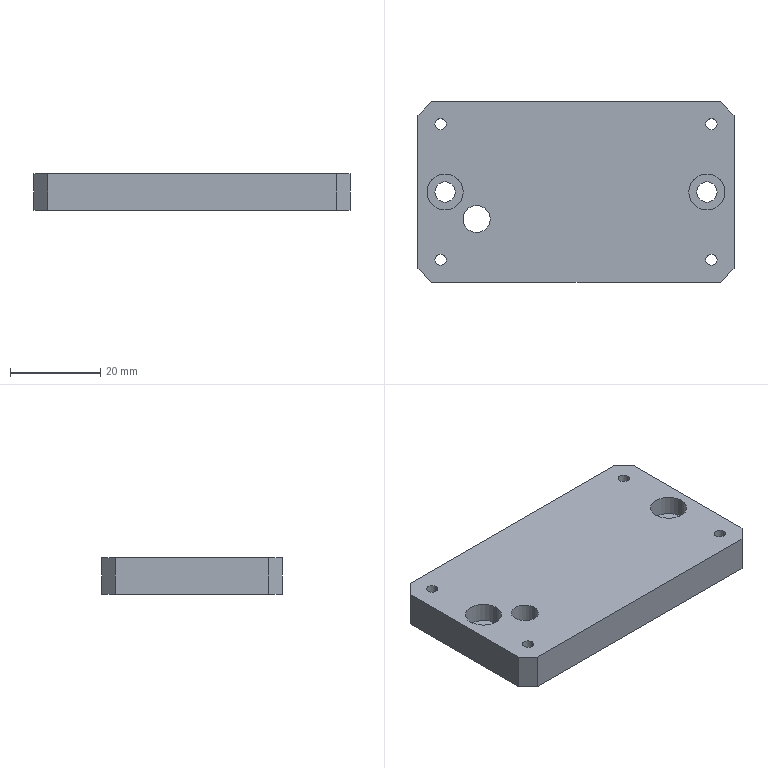Part | STEP file | 11-FG-Z00611 | 1 solid | 36 faces | box 70 x 40 x 8 mm | volume 21065 mm3 | cylinder 22 | plane 14 | commonest cylinder face diameters 2.5 x8 4.5 x4 8 x4 10 x4 6 x2
STEP:
#1=CARTESIAN_POINT('',(-25.,-6.,0.));
#2=VERTEX_POINT('',#1);
#3=CARTESIAN_POINT('',(-19.,-6.,0.));
#4=VERTEX_POINT('',#3);
#5=CARTESIAN_POINT('',(-22.,-6.,0.));
#6=DIRECTION('',(0.,0.,1.));
#7=DIRECTION('',(1.,0.,0.));
#8=AXIS2_PLACEMENT_3D('',#5,#6,#7);
#9=CIRCLE('',#8,3.);
#10=EDGE_CURVE('',#2,#4,#9,.T.);
#11=ORIENTED_EDGE('',*,*,#10,.F.);
#12=CARTESIAN_POINT('',(-25.,-6.,8.));
#13=VERTEX_POINT('',#12);
#14=CARTESIAN_POINT('',(-25.,-6.,-2.));
#15=DIRECTION('',(0.,0.,1.));
#16=VECTOR('',#15,1000.);
#17=LINE('',#14,#16);
#18=EDGE_CURVE('',#2,#13,#17,.T.);
#19=ORIENTED_EDGE('',*,*,#18,.T.);
#20=CARTESIAN_POINT('',(-19.,-6.,8.));
#21=VERTEX_POINT('',#20);
#22=CARTESIAN_POINT('',(-22.,-6.,8.));
#23=DIRECTION('',(0.,0.,1.));
#24=DIRECTION('',(1.,0.,0.));
#25=AXIS2_PLACEMENT_3D('',#22,#23,#24);
#26=CIRCLE('',#25,3.);
#27=EDGE_CURVE('',#13,#21,#26,.T.);
#28=ORIENTED_EDGE('',*,*,#27,.T.);
#29=CARTESIAN_POINT('',(-19.,-6.,-2.));
#30=DIRECTION('',(0.,0.,1.));
#31=VECTOR('',#30,1000.);
#32=LINE('',#29,#31);
#33=EDGE_CURVE('',#4,#21,#32,.T.);
#34=ORIENTED_EDGE('',*,*,#33,.F.);
#35=EDGE_LOOP('',(#11,#19,#28,#34));
#36=FACE_OUTER_BOUND('',#35,.T.);
#37=CARTESIAN_POINT('',(-22.,-6.,-2.));
#38=DIRECTION('',(0.,0.,1.));
#39=DIRECTION('',(1.,0.,0.));
#40=AXIS2_PLACEMENT_3D('',#37,#38,#39);
#41=CYLINDRICAL_SURFACE('',#40,3.);
#42=ADVANCED_FACE('',(#36),#41,.F.);
#43=CARTESIAN_POINT('',(-31.25,15.,0.));
#44=VERTEX_POINT('',#43);
#45=CARTESIAN_POINT('',(-28.75,15.,0.));
#46=VERTEX_POINT('',#45);
#47=CARTESIAN_POINT('',(-30.,15.,0.));
#48=DIRECTION('',(0.,0.,1.));
#49=DIRECTION('',(1.,0.,0.));
#50=AXIS2_PLACEMENT_3D('',#47,#48,#49);
#51=CIRCLE('',#50,1.25);
#52=EDGE_CURVE('',#44,#46,#51,.T.);
#53=ORIENTED_EDGE('',*,*,#52,.F.);
#54=CARTESIAN_POINT('',(-31.25,15.,8.));
#55=VERTEX_POINT('',#54);
#56=CARTESIAN_POINT('',(-31.25,15.,8.));
#57=DIRECTION('',(0.,0.,1.));
#58=VECTOR('',#57,1000.);
#59=LINE('',#56,#58);
#60=EDGE_CURVE('',#44,#55,#59,.T.);
#61=ORIENTED_EDGE('',*,*,#60,.T.);
#62=CARTESIAN_POINT('',(-28.75,15.,8.));
#63=VERTEX_POINT('',#62);
#64=CARTESIAN_POINT('',(-30.,15.,8.));
#65=DIRECTION('',(0.,0.,1.));
#66=DIRECTION('',(1.,0.,0.));
#67=AXIS2_PLACEMENT_3D('',#64,#65,#66);
#68=CIRCLE('',#67,1.25);
#69=EDGE_CURVE('',#55,#63,#68,.T.);
#70=ORIENTED_EDGE('',*,*,#69,.T.);
#71=CARTESIAN_POINT('',(-28.75,15.,8.));
#72=DIRECTION('',(0.,0.,1.));
#73=VECTOR('',#72,1000.);
#74=LINE('',#71,#73);
#75=EDGE_CURVE('',#46,#63,#74,.T.);
#76=ORIENTED_EDGE('',*,*,#75,.F.);
#77=EDGE_LOOP('',(#53,#61,#70,#76));
#78=FACE_OUTER_BOUND('',#77,.T.);
#79=CARTESIAN_POINT('',(-30.,15.,8.));
#80=DIRECTION('',(0.,0.,1.));
#81=DIRECTION('',(1.,0.,0.));
#82=AXIS2_PLACEMENT_3D('',#79,#80,#81);
#83=CYLINDRICAL_SURFACE('',#82,1.25);
#84=ADVANCED_FACE('',(#78),#83,.F.);
#85=CARTESIAN_POINT('',(-31.25,-15.,0.));
#86=VERTEX_POINT('',#85);
#87=CARTESIAN_POINT('',(-28.75,-15.,0.));
#88=VERTEX_POINT('',#87);
#89=CARTESIAN_POINT('',(-30.,-15.,0.));
#90=DIRECTION('',(0.,0.,1.));
#91=DIRECTION('',(1.,0.,0.));
#92=AXIS2_PLACEMENT_3D('',#89,#90,#91);
#93=CIRCLE('',#92,1.25);
#94=EDGE_CURVE('',#86,#88,#93,.T.);
#95=ORIENTED_EDGE('',*,*,#94,.F.);
#96=CARTESIAN_POINT('',(-31.25,-15.,8.));
#97=VERTEX_POINT('',#96);
#98=CARTESIAN_POINT('',(-31.25,-15.,8.));
#99=DIRECTION('',(0.,0.,1.));
#100=VECTOR('',#99,1000.);
#101=LINE('',#98,#100);
#102=EDGE_CURVE('',#86,#97,#101,.T.);
#103=ORIENTED_EDGE('',*,*,#102,.T.);
#104=CARTESIAN_POINT('',(-28.75,-15.,8.));
#105=VERTEX_POINT('',#104);
#106=CARTESIAN_POINT('',(-30.,-15.,8.));
#107=DIRECTION('',(0.,0.,1.));
#108=DIRECTION('',(1.,0.,0.));
#109=AXIS2_PLACEMENT_3D('',#106,#107,#108);
#110=CIRCLE('',#109,1.25);
#111=EDGE_CURVE('',#97,#105,#110,.T.);
#112=ORIENTED_EDGE('',*,*,#111,.T.);
#113=CARTESIAN_POINT('',(-28.75,-15.,8.));
#114=DIRECTION('',(0.,0.,1.));
#115=VECTOR('',#114,1000.);
#116=LINE('',#113,#115);
#117=EDGE_CURVE('',#88,#105,#116,.T.);
#118=ORIENTED_EDGE('',*,*,#117,.F.);
#119=EDGE_LOOP('',(#95,#103,#112,#118));
#120=FACE_OUTER_BOUND('',#119,.T.);
#121=CARTESIAN_POINT('',(-30.,-15.,8.));
#122=DIRECTION('',(0.,0.,1.));
#123=DIRECTION('',(1.,0.,0.));
#124=AXIS2_PLACEMENT_3D('',#121,#122,#123);
#125=CYLINDRICAL_SURFACE('',#124,1.25);
#126=ADVANCED_FACE('',(#120),#125,.F.);
#127=CARTESIAN_POINT('',(28.75,-15.,0.));
#128=VERTEX_POINT('',#127);
#129=CARTESIAN_POINT('',(31.25,-15.,0.));
#130=VERTEX_POINT('',#129);
#131=CARTESIAN_POINT('',(30.,-15.,0.));
#132=DIRECTION('',(0.,0.,1.));
#133=DIRECTION('',(1.,0.,0.));
#134=AXIS2_PLACEMENT_3D('',#131,#132,#133);
#135=CIRCLE('',#134,1.25);
#136=EDGE_CURVE('',#128,#130,#135,.T.);
#137=ORIENTED_EDGE('',*,*,#136,.F.);
#138=CARTESIAN_POINT('',(28.75,-15.,8.));
#139=VERTEX_POINT('',#138);
#140=CARTESIAN_POINT('',(28.75,-15.,8.));
#141=DIRECTION('',(0.,0.,1.));
#142=VECTOR('',#141,1000.);
#143=LINE('',#140,#142);
#144=EDGE_CURVE('',#128,#139,#143,.T.);
#145=ORIENTED_EDGE('',*,*,#144,.T.);
#146=CARTESIAN_POINT('',(31.25,-15.,8.));
#147=VERTEX_POINT('',#146);
#148=CARTESIAN_POINT('',(30.,-15.,8.));
#149=DIRECTION('',(0.,0.,1.));
#150=DIRECTION('',(1.,0.,0.));
#151=AXIS2_PLACEMENT_3D('',#148,#149,#150);
#152=CIRCLE('',#151,1.25);
#153=EDGE_CURVE('',#139,#147,#152,.T.);
#154=ORIENTED_EDGE('',*,*,#153,.T.);
#155=CARTESIAN_POINT('',(31.25,-15.,8.));
#156=DIRECTION('',(0.,0.,1.));
#157=VECTOR('',#156,1000.);
#158=LINE('',#155,#157);
#159=EDGE_CURVE('',#130,#147,#158,.T.);
#160=ORIENTED_EDGE('',*,*,#159,.F.);
#161=EDGE_LOOP('',(#137,#145,#154,#160));
#162=FACE_OUTER_BOUND('',#161,.T.);
#163=CARTESIAN_POINT('',(30.,-15.,8.));
#164=DIRECTION('',(0.,0.,1.));
#165=DIRECTION('',(1.,0.,0.));
#166=AXIS2_PLACEMENT_3D('',#163,#164,#165);
#167=CYLINDRICAL_SURFACE('',#166,1.25);
#168=ADVANCED_FACE('',(#162),#167,.F.);
#169=CARTESIAN_POINT('',(28.75,15.,0.));
#170=VERTEX_POINT('',#169);
#171=CARTESIAN_POINT('',(31.25,15.,0.));
#172=VERTEX_POINT('',#171);
#173=CARTESIAN_POINT('',(30.,15.,0.));
#174=DIRECTION('',(0.,0.,1.));
#175=DIRECTION('',(1.,0.,0.));
#176=AXIS2_PLACEMENT_3D('',#173,#174,#175);
#177=CIRCLE('',#176,1.25);
#178=EDGE_CURVE('',#170,#172,#177,.T.);
#179=ORIENTED_EDGE('',*,*,#178,.F.);
#180=CARTESIAN_POINT('',(28.75,15.,8.));
#181=VERTEX_POINT('',#180);
#182=CARTESIAN_POINT('',(28.75,15.,8.));
#183=DIRECTION('',(0.,0.,1.));
#184=VECTOR('',#183,1000.);
#185=LINE('',#182,#184);
#186=EDGE_CURVE('',#170,#181,#185,.T.);
#187=ORIENTED_EDGE('',*,*,#186,.T.);
#188=CARTESIAN_POINT('',(31.25,15.,8.));
#189=VERTEX_POINT('',#188);
#190=CARTESIAN_POINT('',(30.,15.,8.));
#191=DIRECTION('',(0.,0.,1.));
#192=DIRECTION('',(1.,0.,0.));
#193=AXIS2_PLACEMENT_3D('',#190,#191,#192);
#194=CIRCLE('',#193,1.25);
#195=EDGE_CURVE('',#181,#189,#194,.T.);
#196=ORIENTED_EDGE('',*,*,#195,.T.);
#197=CARTESIAN_POINT('',(31.25,15.,8.));
#198=DIRECTION('',(0.,0.,1.));
#199=VECTOR('',#198,1000.);
#200=LINE('',#197,#199);
#201=EDGE_CURVE('',#172,#189,#200,.T.);
#202=ORIENTED_EDGE('',*,*,#201,.F.);
#203=EDGE_LOOP('',(#179,#187,#196,#202));
#204=FACE_OUTER_BOUND('',#203,.T.);
#205=CARTESIAN_POINT('',(30.,15.,8.));
#206=DIRECTION('',(0.,0.,1.));
#207=DIRECTION('',(1.,0.,0.));
#208=AXIS2_PLACEMENT_3D('',#205,#206,#207);
#209=CYLINDRICAL_SURFACE('',#208,1.25);
#210=ADVANCED_FACE('',(#204),#209,.F.);
#211=CARTESIAN_POINT('',(34.,0.,2.));
#212=VERTEX_POINT('',#211);
#213=CARTESIAN_POINT('',(24.,0.,2.));
#214=VERTEX_POINT('',#213);
#215=CARTESIAN_POINT('',(29.,0.,2.));
#216=DIRECTION('',(0.,0.,-1.));
#217=DIRECTION('',(-1.,0.,0.));
#218=AXIS2_PLACEMENT_3D('',#215,#216,#217);
#219=CIRCLE('',#218,5.);
#220=EDGE_CURVE('',#212,#214,#219,.T.);
#221=ORIENTED_EDGE('',*,*,#220,.F.);
#222=CARTESIAN_POINT('',(34.,0.,0.));
#223=VERTEX_POINT('',#222);
#224=CARTESIAN_POINT('',(34.,0.,2.));
#225=DIRECTION('',(0.,0.,-1.));
#226=VECTOR('',#225,1000.);
#227=LINE('',#224,#226);
#228=EDGE_CURVE('',#212,#223,#227,.T.);
#229=ORIENTED_EDGE('',*,*,#228,.T.);
#230=CARTESIAN_POINT('',(24.,0.,0.));
#231=VERTEX_POINT('',#230);
#232=CARTESIAN_POINT('',(29.,0.,0.));
#233=DIRECTION('',(0.,0.,-1.));
#234=DIRECTION('',(-1.,0.,0.));
#235=AXIS2_PLACEMENT_3D('',#232,#233,#234);
#236=CIRCLE('',#235,5.);
#237=EDGE_CURVE('',#223,#231,#236,.T.);
#238=ORIENTED_EDGE('',*,*,#237,.T.);
#239=CARTESIAN_POINT('',(24.,0.,2.));
#240=DIRECTION('',(0.,0.,-1.));
#241=VECTOR('',#240,1000.);
#242=LINE('',#239,#241);
#243=EDGE_CURVE('',#214,#231,#242,.T.);
#244=ORIENTED_EDGE('',*,*,#243,.F.);
#245=EDGE_LOOP('',(#221,#229,#238,#244));
#246=FACE_OUTER_BOUND('',#245,.T.);
#247=CARTESIAN_POINT('',(29.,0.,2.));
#248=DIRECTION('',(0.,0.,-1.));
#249=DIRECTION('',(-1.,0.,0.));
#250=AXIS2_PLACEMENT_3D('',#247,#248,#249);
#251=CYLINDRICAL_SURFACE('',#250,5.);
#252=ADVANCED_FACE('',(#246),#251,.F.);
#253=CARTESIAN_POINT('',(-24.,0.,2.));
#254=VERTEX_POINT('',#253);
#255=CARTESIAN_POINT('',(-34.,0.,2.));
#256=VERTEX_POINT('',#255);
#257=CARTESIAN_POINT('',(-29.,0.,2.));
#258=DIRECTION('',(0.,0.,-1.));
#259=DIRECTION('',(-1.,0.,0.));
#260=AXIS2_PLACEMENT_3D('',#257,#258,#259);
#261=CIRCLE('',#260,5.);
#262=EDGE_CURVE('',#254,#256,#261,.T.);
#263=ORIENTED_EDGE('',*,*,#262,.F.);
#264=CARTESIAN_POINT('',(-24.,0.,0.));
#265=VERTEX_POINT('',#264);
#266=CARTESIAN_POINT('',(-24.,0.,2.));
#267=DIRECTION('',(0.,0.,-1.));
#268=VECTOR('',#267,1000.);
#269=LINE('',#266,#268);
#270=EDGE_CURVE('',#254,#265,#269,.T.);
#271=ORIENTED_EDGE('',*,*,#270,.T.);
#272=CARTESIAN_POINT('',(-34.,0.,0.));
#273=VERTEX_POINT('',#272);
#274=CARTESIAN_POINT('',(-29.,0.,0.));
#275=DIRECTION('',(0.,0.,-1.));
#276=DIRECTION('',(-1.,0.,0.));
#277=AXIS2_PLACEMENT_3D('',#274,#275,#276);
#278=CIRCLE('',#277,5.);
#279=EDGE_CURVE('',#265,#273,#278,.T.);
#280=ORIENTED_EDGE('',*,*,#279,.T.);
#281=CARTESIAN_POINT('',(-34.,0.,2.));
#282=DIRECTION('',(0.,0.,-1.));
#283=VECTOR('',#282,1000.);
#284=LINE('',#281,#283);
#285=EDGE_CURVE('',#256,#273,#284,.T.);
#286=ORIENTED_EDGE('',*,*,#285,.F.);
#287=EDGE_LOOP('',(#263,#271,#280,#286));
#288=FACE_OUTER_BOUND('',#287,.T.);
#289=CARTESIAN_POINT('',(-29.,0.,2.));
#290=DIRECTION('',(0.,0.,-1.));
#291=DIRECTION('',(-1.,0.,0.));
#292=AXIS2_PLACEMENT_3D('',#289,#290,#291);
#293=CYLINDRICAL_SURFACE('',#292,5.);
#294=ADVANCED_FACE('',(#288),#293,.F.);
#295=CARTESIAN_POINT('',(-33.,0.,3.6));
#296=VERTEX_POINT('',#295);
#297=CARTESIAN_POINT('',(-25.,0.,3.6));
#298=VERTEX_POINT('',#297);
#299=CARTESIAN_POINT('',(-29.,0.,3.6));
#300=DIRECTION('',(0.,0.,1.));
#301=DIRECTION('',(1.,0.,0.));
#302=AXIS2_PLACEMENT_3D('',#299,#300,#301);
#303=CIRCLE('',#302,4.);
#304=EDGE_CURVE('',#296,#298,#303,.T.);
#305=ORIENTED_EDGE('',*,*,#304,.F.);
#306=CARTESIAN_POINT('',(-33.,0.,8.));
#307=VERTEX_POINT('',#306);
#308=CARTESIAN_POINT('',(-33.,0.,8.));
#309=DIRECTION('',(0.,0.,1.));
#310=VECTOR('',#309,1000.);
#311=LINE('',#308,#310);
#312=EDGE_CURVE('',#296,#307,#311,.T.);
#313=ORIENTED_EDGE('',*,*,#312,.T.);
#314=CARTESIAN_POINT('',(-25.,0.,8.));
#315=VERTEX_POINT('',#314);
#316=CARTESIAN_POINT('',(-29.,0.,8.));
#317=DIRECTION('',(0.,0.,1.));
#318=DIRECTION('',(1.,0.,0.));
#319=AXIS2_PLACEMENT_3D('',#316,#317,#318);
#320=CIRCLE('',#319,4.);
#321=EDGE_CURVE('',#307,#315,#320,.T.);
#322=ORIENTED_EDGE('',*,*,#321,.T.);
#323=CARTESIAN_POINT('',(-25.,0.,8.));
#324=DIRECTION('',(0.,0.,1.));
#325=VECTOR('',#324,1000.);
#326=LINE('',#323,#325);
#327=EDGE_CURVE('',#298,#315,#326,.T.);
#328=ORIENTED_EDGE('',*,*,#327,.F.);
#329=EDGE_LOOP('',(#305,#313,#322,#328));
#330=FACE_OUTER_BOUND('',#329,.T.);
#331=CARTESIAN_POINT('',(-29.,0.,8.));
#332=DIRECTION('',(0.,0.,1.));
#333=DIRECTION('',(1.,0.,0.));
#334=AXIS2_PLACEMENT_3D('',#331,#332,#333);
#335=CYLINDRICAL_SURFACE('',#334,4.);
#336=ADVANCED_FACE('',(#330),#335,.F.);
#337=CARTESIAN_POINT('',(25.,0.,3.6));
#338=VERTEX_POINT('',#337);
#339=CARTESIAN_POINT('',(33.,0.,3.6));
#340=VERTEX_POINT('',#339);
#341=CARTESIAN_POINT('',(29.,0.,3.6));
#342=DIRECTION('',(0.,0.,1.));
#343=DIRECTION('',(1.,0.,0.));
#344=AXIS2_PLACEMENT_3D('',#341,#342,#343);
#345=CIRCLE('',#344,4.);
#346=EDGE_CURVE('',#338,#340,#345,.T.);
#347=ORIENTED_EDGE('',*,*,#346,.F.);
#348=CARTESIAN_POINT('',(25.,0.,8.));
#349=VERTEX_POINT('',#348);
#350=CARTESIAN_POINT('',(25.,0.,8.));
#351=DIRECTION('',(0.,0.,1.));
#352=VECTOR('',#351,1000.);
#353=LINE('',#350,#352);
#354=EDGE_CURVE('',#338,#349,#353,.T.);
#355=ORIENTED_EDGE('',*,*,#354,.T.);
#356=CARTESIAN_POINT('',(33.,0.,8.));
#357=VERTEX_POINT('',#356);
#358=CARTESIAN_POINT('',(29.,0.,8.));
#359=DIRECTION('',(0.,0.,1.));
#360=DIRECTION('',(1.,0.,0.));
#361=AXIS2_PLACEMENT_3D('',#358,#359,#360);
#362=CIRCLE('',#361,4.);
#363=EDGE_CURVE('',#349,#357,#362,.T.);
#364=ORIENTED_EDGE('',*,*,#363,.T.);
#365=CARTESIAN_POINT('',(33.,0.,8.));
#366=DIRECTION('',(0.,0.,1.));
#367=VECTOR('',#366,1000.);
#368=LINE('',#365,#367);
#369=EDGE_CURVE('',#340,#357,#368,.T.);
#370=ORIENTED_EDGE('',*,*,#369,.F.);
#371=EDGE_LOOP('',(#347,#355,#364,#370));
#372=FACE_OUTER_BOUND('',#371,.T.);
#373=CARTESIAN_POINT('',(29.,0.,8.));
#374=DIRECTION('',(0.,0.,1.));
#375=DIRECTION('',(1.,0.,0.));
#376=AXIS2_PLACEMENT_3D('',#373,#374,#375);
#377=CYLINDRICAL_SURFACE('',#376,4.);
#378=ADVANCED_FACE('',(#372),#377,.F.);
#379=CARTESIAN_POINT('',(-31.25,0.,2.));
#380=VERTEX_POINT('',#379);
#381=CARTESIAN_POINT('',(-26.75,0.,2.));
#382=VERTEX_POINT('',#381);
#383=CARTESIAN_POINT('',(-29.,0.,2.));
#384=DIRECTION('',(0.,0.,1.));
#385=DIRECTION('',(-1.,0.,0.));
#386=AXIS2_PLACEMENT_3D('',#383,#384,#385);
#387=CIRCLE('',#386,2.25);
#388=EDGE_CURVE('',#380,#382,#387,.T.);
#389=ORIENTED_EDGE('',*,*,#388,.F.);
#390=CARTESIAN_POINT('',(-31.25,0.,3.6));
#391=VERTEX_POINT('',#390);
#392=CARTESIAN_POINT('',(-31.25,0.,8.));
#393=DIRECTION('',(0.,0.,1.));
#394=VECTOR('',#393,1000.);
#395=LINE('',#392,#394);
#396=EDGE_CURVE('',#380,#391,#395,.T.);
#397=ORIENTED_EDGE('',*,*,#396,.T.);
#398=CARTESIAN_POINT('',(-26.75,0.,3.6));
#399=VERTEX_POINT('',#398);
#400=CARTESIAN_POINT('',(-29.,0.,3.6));
#401=DIRECTION('',(0.,0.,1.));
#402=DIRECTION('',(1.,0.,0.));
#403=AXIS2_PLACEMENT_3D('',#400,#401,#402);
#404=CIRCLE('',#403,2.25);
#405=EDGE_CURVE('',#391,#399,#404,.T.);
#406=ORIENTED_EDGE('',*,*,#405,.T.);
#407=CARTESIAN_POINT('',(-26.75,0.,8.));
#408=DIRECTION('',(0.,0.,1.));
#409=VECTOR('',#408,1000.);
#410=LINE('',#407,#409);
#411=EDGE_CURVE('',#382,#399,#410,.T.);
#412=ORIENTED_EDGE('',*,*,#411,.F.);
#413=EDGE_LOOP('',(#389,#397,#406,#412));
#414=FACE_OUTER_BOUND('',#413,.T.);
#415=CARTESIAN_POINT('',(-29.,0.,8.));
#416=DIRECTION('',(0.,0.,1.));
#417=DIRECTION('',(1.,0.,0.));
#418=AXIS2_PLACEMENT_3D('',#415,#416,#417);
#419=CYLINDRICAL_SURFACE('',#418,2.25);
#420=ADVANCED_FACE('',(#414),#419,.F.);
#421=CARTESIAN_POINT('',(26.75,0.,2.));
#422=VERTEX_POINT('',#421);
#423=CARTESIAN_POINT('',(31.25,0.,2.));
#424=VERTEX_POINT('',#423);
#425=CARTESIAN_POINT('',(29.,0.,2.));
#426=DIRECTION('',(0.,0.,1.));
#427=DIRECTION('',(-1.,0.,0.));
#428=AXIS2_PLACEMENT_3D('',#425,#426,#427);
#429=CIRCLE('',#428,2.25);
#430=EDGE_CURVE('',#422,#424,#429,.T.);
#431=ORIENTED_EDGE('',*,*,#430,.F.);
#432=CARTESIAN_POINT('',(26.75,0.,3.6));
#433=VERTEX_POINT('',#432);
#434=CARTESIAN_POINT('',(26.75,0.,8.));
#435=DIRECTION('',(0.,0.,1.));
#436=VECTOR('',#435,1000.);
#437=LINE('',#434,#436);
#438=EDGE_CURVE('',#422,#433,#437,.T.);
#439=ORIENTED_EDGE('',*,*,#438,.T.);
#440=CARTESIAN_POINT('',(31.25,0.,3.6));
#441=VERTEX_POINT('',#440);
#442=CARTESIAN_POINT('',(29.,0.,3.6));
#443=DIRECTION('',(0.,0.,1.));
#444=DIRECTION('',(1.,0.,0.));
#445=AXIS2_PLACEMENT_3D('',#442,#443,#444);
#446=CIRCLE('',#445,2.25);
#447=EDGE_CURVE('',#433,#441,#446,.T.);
#448=ORIENTED_EDGE('',*,*,#447,.T.);
#449=CARTESIAN_POINT('',(31.25,0.,8.));
#450=DIRECTION('',(0.,0.,1.));
#451=VECTOR('',#450,1000.);
#452=LINE('',#449,#451);
#453=EDGE_CURVE('',#424,#441,#452,.T.);
#454=ORIENTED_EDGE('',*,*,#453,.F.);
#455=EDGE_LOOP('',(#431,#439,#448,#454));
#456=FACE_OUTER_BOUND('',#455,.T.);
#457=CARTESIAN_POINT('',(29.,0.,8.));
#458=DIRECTION('',(0.,0.,1.));
#459=DIRECTION('',(1.,0.,0.));
#460=AXIS2_PLACEMENT_3D('',#457,#458,#459);
#461=CYLINDRICAL_SURFACE('',#460,2.25);
#462=ADVANCED_FACE('',(#456),#461,.F.);
#463=ORIENTED_EDGE('',*,*,#438,.F.);
#464=CARTESIAN_POINT('',(29.,0.,2.));
#465=DIRECTION('',(0.,0.,1.));
#466=DIRECTION('',(-1.,0.,0.));
#467=AXIS2_PLACEMENT_3D('',#464,#465,#466);
#468=CIRCLE('',#467,2.25);
#469=EDGE_CURVE('',#424,#422,#468,.T.);
#470=ORIENTED_EDGE('',*,*,#469,.F.);
#471=ORIENTED_EDGE('',*,*,#453,.T.);
#472=CARTESIAN_POINT('',(29.,0.,3.6));
#473=DIRECTION('',(0.,0.,1.));
#474=DIRECTION('',(1.,0.,0.));
#475=AXIS2_PLACEMENT_3D('',#472,#473,#474);
#476=CIRCLE('',#475,2.25);
#477=EDGE_CURVE('',#441,#433,#476,.T.);
#478=ORIENTED_EDGE('',*,*,#477,.T.);
#479=EDGE_LOOP('',(#463,#470,#471,#478));
#480=FACE_OUTER_BOUND('',#479,.T.);
#481=CARTESIAN_POINT('',(29.,0.,8.));
#482=DIRECTION('',(0.,0.,1.));
#483=DIRECTION('',(1.,0.,0.));
#484=AXIS2_PLACEMENT_3D('',#481,#482,#483);
#485=CYLINDRICAL_SURFACE('',#484,2.25);
#486=ADVANCED_FACE('',(#480),#485,.F.);
#487=ORIENTED_EDGE('',*,*,#396,.F.);
#488=CARTESIAN_POINT('',(-29.,0.,2.));
#489=DIRECTION('',(0.,0.,1.));
#490=DIRECTION('',(-1.,0.,0.));
#491=AXIS2_PLACEMENT_3D('',#488,#489,#490);
#492=CIRCLE('',#491,2.25);
#493=EDGE_CURVE('',#382,#380,#492,.T.);
#494=ORIENTED_EDGE('',*,*,#493,.F.);
#495=ORIENTED_EDGE('',*,*,#411,.T.);
#496=CARTESIAN_POINT('',(-29.,0.,3.6));
#497=DIRECTION('',(0.,0.,1.));
#498=DIRECTION('',(1.,0.,0.));
#499=AXIS2_PLACEMENT_3D('',#496,#497,#498);
#500=CIRCLE('',#499,2.25);
#501=EDGE_CURVE('',#399,#391,#500,.T.);
#502=ORIENTED_EDGE('',*,*,#501,.T.);
#503=EDGE_LOOP('',(#487,#494,#495,#502));
#504=FACE_OUTER_BOUND('',#503,.T.);
#505=CARTESIAN_POINT('',(-29.,0.,8.));
#506=DIRECTION('',(0.,0.,1.));
#507=DIRECTION('',(1.,0.,0.));
#508=AXIS2_PLACEMENT_3D('',#505,#506,#507);
#509=CYLINDRICAL_SURFACE('',#508,2.25);
#510=ADVANCED_FACE('',(#504),#509,.F.);
#511=CARTESIAN_POINT('',(35.,-17.,8.));
#512=VERTEX_POINT('',#511);
#513=CARTESIAN_POINT('',(35.,17.,8.));
#514=VERTEX_POINT('',#513);
#515=CARTESIAN_POINT('',(35.,20.,8.));
#516=DIRECTION('',(0.,1.,0.));
#517=VECTOR('',#516,1000.);
#518=LINE('',#515,#517);
#519=EDGE_CURVE('',#512,#514,#518,.T.);
#520=ORIENTED_EDGE('',*,*,#519,.F.);
#521=CARTESIAN_POINT('',(35.,-17.,0.));
#522=VERTEX_POINT('',#521);
#523=CARTESIAN_POINT('',(35.,-17.,8.));
#524=DIRECTION('',(0.,0.,-1.));
#525=VECTOR('',#524,1000.);
#526=LINE('',#523,#525);
#527=EDGE_CURVE('',#512,#522,#526,.T.);
#528=ORIENTED_EDGE('',*,*,#527,.T.);
#529=CARTESIAN_POINT('',(35.,17.,0.));
#530=VERTEX_POINT('',#529);
#531=CARTESIAN_POINT('',(35.,20.,0.));
#532=DIRECTION('',(0.,1.,0.));
#533=VECTOR('',#532,1000.);
#534=LINE('',#531,#533);
#535=EDGE_CURVE('',#522,#530,#534,.T.);
#536=ORIENTED_EDGE('',*,*,#535,.T.);
#537=CARTESIAN_POINT('',(35.,17.,8.));
#538=DIRECTION('',(0.,0.,1.));
#539=VECTOR('',#538,1000.);
#540=LINE('',#537,#539);
#541=EDGE_CURVE('',#530,#514,#540,.T.);
#542=ORIENTED_EDGE('',*,*,#541,.T.);
#543=EDGE_LOOP('',(#520,#528,#536,#542));
#544=FACE_OUTER_BOUND('',#543,.T.);
#545=CARTESIAN_POINT('',(35.,20.,8.));
#546=DIRECTION('',(-1.,0.,0.));
#547=DIRECTION('',(0.,-1.,0.));
#548=AXIS2_PLACEMENT_3D('',#545,#546,#547);
#549=PLANE('',#548);
#550=ADVANCED_FACE('',(#544),#549,.F.);
#551=CARTESIAN_POINT('',(32.,20.,8.));
#552=VERTEX_POINT('',#551);
#553=CARTESIAN_POINT('',(-32.,20.,8.));
#554=VERTEX_POINT('',#553);
#555=CARTESIAN_POINT('',(-35.,20.,8.));
#556=DIRECTION('',(-1.,0.,0.));
#557=VECTOR('',#556,1000.);
#558=LINE('',#555,#557);
#559=EDGE_CURVE('',#552,#554,#558,.T.);
#560=ORIENTED_EDGE('',*,*,#559,.F.);
#561=CARTESIAN_POINT('',(32.,20.,0.));
#562=VERTEX_POINT('',#561);
#563=CARTESIAN_POINT('',(32.,20.,8.));
#564=DIRECTION('',(0.,0.,-1.));
#565=VECTOR('',#564,1000.);
#566=LINE('',#563,#565);
#567=EDGE_CURVE('',#552,#562,#566,.T.);
#568=ORIENTED_EDGE('',*,*,#567,.T.);
#569=CARTESIAN_POINT('',(-32.,20.,0.));
#570=VERTEX_POINT('',#569);
#571=CARTESIAN_POINT('',(-35.,20.,0.));
#572=DIRECTION('',(-1.,0.,0.));
#573=VECTOR('',#572,1000.);
#574=LINE('',#571,#573);
#575=EDGE_CURVE('',#562,#570,#574,.T.);
#576=ORIENTED_EDGE('',*,*,#575,.T.);
#577=CARTESIAN_POINT('',(-32.,20.,8.));
#578=DIRECTION('',(0.,0.,1.));
#579=VECTOR('',#578,1000.);
#580=LINE('',#577,#579);
#581=EDGE_CURVE('',#570,#554,#580,.T.);
#582=ORIENTED_EDGE('',*,*,#581,.T.);
#583=EDGE_LOOP('',(#560,#568,#576,#582));
#584=FACE_OUTER_BOUND('',#583,.T.);
#585=CARTESIAN_POINT('',(-35.,20.,8.));
#586=DIRECTION('',(0.,-1.,0.));
#587=DIRECTION('',(0.,0.,-1.));
#588=AXIS2_PLACEMENT_3D('',#585,#586,#587);
#589=PLANE('',#588);
#590=ADVANCED_FACE('',(#584),#589,.F.);
#591=CARTESIAN_POINT('',(-35.,17.,0.));
#592=VERTEX_POINT('',#591);
#593=CARTESIAN_POINT('',(-35.,-17.,0.));
#594=VERTEX_POINT('',#593);
#595=CARTESIAN_POINT('',(-35.,20.,0.));
#596=DIRECTION('',(0.,-1.,0.));
#597=VECTOR('',#596,1000.);
#598=LINE('',#595,#597);
#599=EDGE_CURVE('',#592,#594,#598,.T.);
#600=ORIENTED_EDGE('',*,*,#599,.T.);
#601=CARTESIAN_POINT('',(-35.,-17.,8.));
#602=VERTEX_POINT('',#601);
#603=CARTESIAN_POINT('',(-35.,-17.,8.));
#604=DIRECTION('',(0.,0.,1.));
#605=VECTOR('',#604,1000.);
#606=LINE('',#603,#605);
#607=EDGE_CURVE('',#594,#602,#606,.T.);
#608=ORIENTED_EDGE('',*,*,#607,.T.);
#609=CARTESIAN_POINT('',(-35.,17.,8.));
#610=VERTEX_POINT('',#609);
#611=CARTESIAN_POINT('',(-35.,20.,8.));
#612=DIRECTION('',(0.,-1.,0.));
#613=VECTOR('',#612,1000.);
#614=LINE('',#611,#613);
#615=EDGE_CURVE('',#610,#602,#614,.T.);
#616=ORIENTED_EDGE('',*,*,#615,.F.);
#617=CARTESIAN_POINT('',(-35.,17.,8.));
#618=DIRECTION('',(0.,0.,-1.));
#619=VECTOR('',#618,1000.);
#620=LINE('',#617,#619);
#621=EDGE_CURVE('',#610,#592,#620,.T.);
#622=ORIENTED_EDGE('',*,*,#621,.T.);
#623=EDGE_LOOP('',(#600,#608,#616,#622));
#624=FACE_OUTER_BOUND('',#623,.T.);
#625=CARTESIAN_POINT('',(-35.,20.,8.));
#626=DIRECTION('',(1.,0.,0.));
#627=DIRECTION('',(0.,1.,0.));
#628=AXIS2_PLACEMENT_3D('',#625,#626,#627);
#629=PLANE('',#628);
#630=ADVANCED_FACE('',(#624),#629,.F.);
#631=CARTESIAN_POINT('',(-32.,-20.,0.));
#632=VERTEX_POINT('',#631);
#633=CARTESIAN_POINT('',(32.,-20.,0.));
#634=VERTEX_POINT('',#633);
#635=CARTESIAN_POINT('',(-35.,-20.,0.));
#636=DIRECTION('',(1.,0.,0.));
#637=VECTOR('',#636,1000.);
#638=LINE('',#635,#637);
#639=EDGE_CURVE('',#632,#634,#638,.T.);
#640=ORIENTED_EDGE('',*,*,#639,.T.);
#641=CARTESIAN_POINT('',(32.,-20.,8.));
#642=VERTEX_POINT('',#641);
#643=CARTESIAN_POINT('',(32.,-20.,8.));
#644=DIRECTION('',(0.,0.,1.));
#645=VECTOR('',#644,1000.);
#646=LINE('',#643,#645);
#647=EDGE_CURVE('',#634,#642,#646,.T.);
#648=ORIENTED_EDGE('',*,*,#647,.T.);
#649=CARTESIAN_POINT('',(-32.,-20.,8.));
#650=VERTEX_POINT('',#649);
#651=CARTESIAN_POINT('',(-35.,-20.,8.));
#652=DIRECTION('',(1.,0.,0.));
#653=VECTOR('',#652,1000.);
#654=LINE('',#651,#653);
#655=EDGE_CURVE('',#650,#642,#654,.T.);
#656=ORIENTED_EDGE('',*,*,#655,.F.);
#657=CARTESIAN_POINT('',(-32.,-20.,8.));
#658=DIRECTION('',(0.,0.,-1.));
#659=VECTOR('',#658,1000.);
#660=LINE('',#657,#659);
#661=EDGE_CURVE('',#650,#632,#660,.T.);
#662=ORIENTED_EDGE('',*,*,#661,.T.);
#663=EDGE_LOOP('',(#640,#648,#656,#662));
#664=FACE_OUTER_BOUND('',#663,.T.);
#665=CARTESIAN_POINT('',(-35.,-20.,8.));
#666=DIRECTION('',(0.,1.,0.));
#667=DIRECTION('',(0.,0.,1.));
#668=AXIS2_PLACEMENT_3D('',#665,#666,#667);
#669=PLANE('',#668);
#670=ADVANCED_FACE('',(#664),#669,.F.);
#671=CARTESIAN_POINT('',(-22.,-6.,8.));
#672=DIRECTION('',(0.,0.,1.));
#673=DIRECTION('',(1.,0.,0.));
#674=AXIS2_PLACEMENT_3D('',#671,#672,#673);
#675=CIRCLE('',#674,3.);
#676=EDGE_CURVE('',#21,#13,#675,.T.);
#677=ORIENTED_EDGE('',*,*,#676,.F.);
#678=ORIENTED_EDGE('',*,*,#27,.F.);
#679=EDGE_LOOP('',(#677,#678));
#680=FACE_BOUND('',#679,.T.);
#681=CARTESIAN_POINT('',(-30.,15.,8.));
#682=DIRECTION('',(0.,0.,1.));
#683=DIRECTION('',(1.,0.,0.));
#684=AXIS2_PLACEMENT_3D('',#681,#682,#683);
#685=CIRCLE('',#684,1.25);
#686=EDGE_CURVE('',#63,#55,#685,.T.);
#687=ORIENTED_EDGE('',*,*,#686,.F.);
#688=ORIENTED_EDGE('',*,*,#69,.F.);
#689=EDGE_LOOP('',(#687,#688));
#690=FACE_BOUND('',#689,.T.);
#691=CARTESIAN_POINT('',(-30.,-15.,8.));
#692=DIRECTION('',(0.,0.,1.));
#693=DIRECTION('',(1.,0.,0.));
#694=AXIS2_PLACEMENT_3D('',#691,#692,#693);
#695=CIRCLE('',#694,1.25);
#696=EDGE_CURVE('',#105,#97,#695,.T.);
#697=ORIENTED_EDGE('',*,*,#696,.F.);
#698=ORIENTED_EDGE('',*,*,#111,.F.);
#699=EDGE_LOOP('',(#697,#698));
#700=FACE_BOUND('',#699,.T.);
#701=CARTESIAN_POINT('',(30.,-15.,8.));
#702=DIRECTION('',(0.,0.,1.));
#703=DIRECTION('',(1.,0.,0.));
#704=AXIS2_PLACEMENT_3D('',#701,#702,#703);
#705=CIRCLE('',#704,1.25);
#706=EDGE_CURVE('',#147,#139,#705,.T.);
#707=ORIENTED_EDGE('',*,*,#706,.F.);
#708=ORIENTED_EDGE('',*,*,#153,.F.);
#709=EDGE_LOOP('',(#707,#708));
#710=FACE_BOUND('',#709,.T.);
#711=CARTESIAN_POINT('',(30.,15.,8.));
#712=DIRECTION('',(0.,0.,1.));
#713=DIRECTION('',(1.,0.,0.));
#714=AXIS2_PLACEMENT_3D('',#711,#712,#713);
#715=CIRCLE('',#714,1.25);
#716=EDGE_CURVE('',#189,#181,#715,.T.);
#717=ORIENTED_EDGE('',*,*,#716,.F.);
#718=ORIENTED_EDGE('',*,*,#195,.F.);
#719=EDGE_LOOP('',(#717,#718));
#720=FACE_BOUND('',#719,.T.);
#721=CARTESIAN_POINT('',(-29.,0.,8.));
#722=DIRECTION('',(0.,0.,1.));
#723=DIRECTION('',(1.,0.,0.));
#724=AXIS2_PLACEMENT_3D('',#721,#722,#723);
#725=CIRCLE('',#724,4.);
#726=EDGE_CURVE('',#315,#307,#725,.T.);
#727=ORIENTED_EDGE('',*,*,#726,.F.);
#728=ORIENTED_EDGE('',*,*,#321,.F.);
#729=EDGE_LOOP('',(#727,#728));
#730=FACE_BOUND('',#729,.T.);
#731=CARTESIAN_POINT('',(29.,0.,8.));
#732=DIRECTION('',(0.,0.,1.));
#733=DIRECTION('',(1.,0.,0.));
#734=AXIS2_PLACEMENT_3D('',#731,#732,#733);
#735=CIRCLE('',#734,4.);
#736=EDGE_CURVE('',#357,#349,#735,.T.);
#737=ORIENTED_EDGE('',*,*,#736,.F.);
#738=ORIENTED_EDGE('',*,*,#363,.F.);
#739=EDGE_LOOP('',(#737,#738));
#740=FACE_BOUND('',#739,.T.);
#741=ORIENTED_EDGE('',*,*,#655,.T.);
#742=CARTESIAN_POINT('',(26.,-26.,8.));
#743=DIRECTION('',(0.7071,0.7071,0.));
#744=VECTOR('',#743,1000.);
#745=LINE('',#742,#744);
#746=EDGE_CURVE('',#642,#512,#745,.T.);
#747=ORIENTED_EDGE('',*,*,#746,.T.);
#748=ORIENTED_EDGE('',*,*,#519,.T.);
#749=CARTESIAN_POINT('',(26.,26.,8.));
#750=DIRECTION('',(-0.7071,0.7071,0.));
#751=VECTOR('',#750,1000.);
#752=LINE('',#749,#751);
#753=EDGE_CURVE('',#514,#552,#752,.T.);
#754=ORIENTED_EDGE('',*,*,#753,.T.);
#755=ORIENTED_EDGE('',*,*,#559,.T.);
#756=CARTESIAN_POINT('',(-26.,26.,8.));
#757=DIRECTION('',(-0.7071,-0.7071,0.));
#758=VECTOR('',#757,1000.);
#759=LINE('',#756,#758);
#760=EDGE_CURVE('',#554,#610,#759,.T.);
#761=ORIENTED_EDGE('',*,*,#760,.T.);
#762=ORIENTED_EDGE('',*,*,#615,.T.);
#763=CARTESIAN_POINT('',(-26.,-26.,8.));
#764=DIRECTION('',(0.7071,-0.7071,0.));
#765=VECTOR('',#764,1000.);
#766=LINE('',#763,#765);
#767=EDGE_CURVE('',#602,#650,#766,.T.);
#768=ORIENTED_EDGE('',*,*,#767,.T.);
#769=EDGE_LOOP('',(#741,#747,#748,#754,#755,#761,#762,#768));
#770=FACE_OUTER_BOUND('',#769,.T.);
#771=CARTESIAN_POINT('',(0.,0.,8.));
#772=DIRECTION('',(0.,0.,1.));
#773=DIRECTION('',(1.,0.,0.));
#774=AXIS2_PLACEMENT_3D('',#771,#772,#773);
#775=PLANE('',#774);
#776=ADVANCED_FACE('',(#680,#690,#700,#710,#720,#730,#740,#770),#775,.T.);
#777=CARTESIAN_POINT('',(-22.,-6.,0.));
#778=DIRECTION('',(0.,0.,1.));
#779=DIRECTION('',(1.,0.,0.));
#780=AXIS2_PLACEMENT_3D('',#777,#778,#779);
#781=CIRCLE('',#780,3.);
#782=EDGE_CURVE('',#4,#2,#781,.T.);
#783=ORIENTED_EDGE('',*,*,#782,.T.);
#784=ORIENTED_EDGE('',*,*,#10,.T.);
#785=EDGE_LOOP('',(#783,#784));
#786=FACE_BOUND('',#785,.T.);
#787=CARTESIAN_POINT('',(-30.,15.,0.));
#788=DIRECTION('',(0.,0.,1.));
#789=DIRECTION('',(1.,0.,0.));
#790=AXIS2_PLACEMENT_3D('',#787,#788,#789);
#791=CIRCLE('',#790,1.25);
#792=EDGE_CURVE('',#46,#44,#791,.T.);
#793=ORIENTED_EDGE('',*,*,#792,.T.);
#794=ORIENTED_EDGE('',*,*,#52,.T.);
#795=EDGE_LOOP('',(#793,#794));
#796=FACE_BOUND('',#795,.T.);
#797=CARTESIAN_POINT('',(-30.,-15.,0.));
#798=DIRECTION('',(0.,0.,1.));
#799=DIRECTION('',(1.,0.,0.));
#800=AXIS2_PLACEMENT_3D('',#797,#798,#799);
#801=CIRCLE('',#800,1.25);
#802=EDGE_CURVE('',#88,#86,#801,.T.);
#803=ORIENTED_EDGE('',*,*,#802,.T.);
#804=ORIENTED_EDGE('',*,*,#94,.T.);
#805=EDGE_LOOP('',(#803,#804));
#806=FACE_BOUND('',#805,.T.);
#807=CARTESIAN_POINT('',(30.,-15.,0.));
#808=DIRECTION('',(0.,0.,1.));
#809=DIRECTION('',(1.,0.,0.));
#810=AXIS2_PLACEMENT_3D('',#807,#808,#809);
#811=CIRCLE('',#810,1.25);
#812=EDGE_CURVE('',#130,#128,#811,.T.);
#813=ORIENTED_EDGE('',*,*,#812,.T.);
#814=ORIENTED_EDGE('',*,*,#136,.T.);
#815=EDGE_LOOP('',(#813,#814));
#816=FACE_BOUND('',#815,.T.);
#817=CARTESIAN_POINT('',(30.,15.,0.));
#818=DIRECTION('',(0.,0.,1.));
#819=DIRECTION('',(1.,0.,0.));
#820=AXIS2_PLACEMENT_3D('',#817,#818,#819);
#821=CIRCLE('',#820,1.25);
#822=EDGE_CURVE('',#172,#170,#821,.T.);
#823=ORIENTED_EDGE('',*,*,#822,.T.);
#824=ORIENTED_EDGE('',*,*,#178,.T.);
#825=EDGE_LOOP('',(#823,#824));
#826=FACE_BOUND('',#825,.T.);
#827=CARTESIAN_POINT('',(29.,0.,0.));
#828=DIRECTION('',(0.,0.,-1.));
#829=DIRECTION('',(-1.,0.,0.));
#830=AXIS2_PLACEMENT_3D('',#827,#828,#829);
#831=CIRCLE('',#830,5.);
#832=EDGE_CURVE('',#231,#223,#831,.T.);
#833=ORIENTED_EDGE('',*,*,#832,.F.);
#834=ORIENTED_EDGE('',*,*,#237,.F.);
#835=EDGE_LOOP('',(#833,#834));
#836=FACE_BOUND('',#835,.T.);
#837=CARTESIAN_POINT('',(-29.,0.,0.));
#838=DIRECTION('',(0.,0.,-1.));
#839=DIRECTION('',(-1.,0.,0.));
#840=AXIS2_PLACEMENT_3D('',#837,#838,#839);
#841=CIRCLE('',#840,5.);
#842=EDGE_CURVE('',#273,#265,#841,.T.);
#843=ORIENTED_EDGE('',*,*,#842,.F.);
#844=ORIENTED_EDGE('',*,*,#279,.F.);
#845=EDGE_LOOP('',(#843,#844));
#846=FACE_BOUND('',#845,.T.);
#847=ORIENTED_EDGE('',*,*,#535,.F.);
#848=CARTESIAN_POINT('',(35.,-17.,0.));
#849=DIRECTION('',(-0.7071,-0.7071,0.));
#850=VECTOR('',#849,1000.);
#851=LINE('',#848,#850);
#852=EDGE_CURVE('',#522,#634,#851,.T.);
#853=ORIENTED_EDGE('',*,*,#852,.T.);
#854=ORIENTED_EDGE('',*,*,#639,.F.);
#855=CARTESIAN_POINT('',(-32.,-20.,0.));
#856=DIRECTION('',(-0.7071,0.7071,0.));
#857=VECTOR('',#856,1000.);
#858=LINE('',#855,#857);
#859=EDGE_CURVE('',#632,#594,#858,.T.);
#860=ORIENTED_EDGE('',*,*,#859,.T.);
#861=ORIENTED_EDGE('',*,*,#599,.F.);
#862=CARTESIAN_POINT('',(-35.,17.,0.));
#863=DIRECTION('',(0.7071,0.7071,0.));
#864=VECTOR('',#863,1000.);
#865=LINE('',#862,#864);
#866=EDGE_CURVE('',#592,#570,#865,.T.);
#867=ORIENTED_EDGE('',*,*,#866,.T.);
#868=ORIENTED_EDGE('',*,*,#575,.F.);
#869=CARTESIAN_POINT('',(32.,20.,0.));
#870=DIRECTION('',(0.7071,-0.7071,0.));
#871=VECTOR('',#870,1000.);
#872=LINE('',#869,#871);
#873=EDGE_CURVE('',#562,#530,#872,.T.);
#874=ORIENTED_EDGE('',*,*,#873,.T.);
#875=EDGE_LOOP('',(#847,#853,#854,#860,#861,#867,#868,#874));
#876=FACE_OUTER_BOUND('',#875,.T.);
#877=CARTESIAN_POINT('',(0.,0.,0.));
#878=DIRECTION('',(0.,0.,1.));
#879=DIRECTION('',(1.,0.,0.));
#880=AXIS2_PLACEMENT_3D('',#877,#878,#879);
#881=PLANE('',#880);
#882=ADVANCED_FACE('',(#786,#796,#806,#816,#826,#836,#846,#876),#881,.F.);
#883=ORIENTED_EDGE('',*,*,#746,.F.);
#884=ORIENTED_EDGE('',*,*,#647,.F.);
#885=ORIENTED_EDGE('',*,*,#852,.F.);
#886=ORIENTED_EDGE('',*,*,#527,.F.);
#887=EDGE_LOOP('',(#883,#884,#885,#886));
#888=FACE_OUTER_BOUND('',#887,.T.);
#889=CARTESIAN_POINT('',(35.,-17.,8.));
#890=DIRECTION('',(-0.7071,0.7071,0.));
#891=DIRECTION('',(0.,0.,-1.));
#892=AXIS2_PLACEMENT_3D('',#889,#890,#891);
#893=PLANE('',#892);
#894=ADVANCED_FACE('',(#888),#893,.F.);
#895=ORIENTED_EDGE('',*,*,#753,.F.);
#896=ORIENTED_EDGE('',*,*,#541,.F.);
#897=ORIENTED_EDGE('',*,*,#873,.F.);
#898=ORIENTED_EDGE('',*,*,#567,.F.);
#899=EDGE_LOOP('',(#895,#896,#897,#898));
#900=FACE_OUTER_BOUND('',#899,.T.);
#901=CARTESIAN_POINT('',(32.,20.,8.));
#902=DIRECTION('',(-0.7071,-0.7071,0.));
#903=DIRECTION('',(0.,0.,-1.));
#904=AXIS2_PLACEMENT_3D('',#901,#902,#903);
#905=PLANE('',#904);
#906=ADVANCED_FACE('',(#900),#905,.F.);
#907=ORIENTED_EDGE('',*,*,#767,.F.);
#908=ORIENTED_EDGE('',*,*,#607,.F.);
#909=ORIENTED_EDGE('',*,*,#859,.F.);
#910=ORIENTED_EDGE('',*,*,#661,.F.);
#911=EDGE_LOOP('',(#907,#908,#909,#910));
#912=FACE_OUTER_BOUND('',#911,.T.);
#913=CARTESIAN_POINT('',(-32.,-20.,8.));
#914=DIRECTION('',(0.7071,0.7071,0.));
#915=DIRECTION('',(0.,0.,-1.));
#916=AXIS2_PLACEMENT_3D('',#913,#914,#915);
#917=PLANE('',#916);
#918=ADVANCED_FACE('',(#912),#917,.F.);
#919=ORIENTED_EDGE('',*,*,#760,.F.);
#920=ORIENTED_EDGE('',*,*,#581,.F.);
#921=ORIENTED_EDGE('',*,*,#866,.F.);
#922=ORIENTED_EDGE('',*,*,#621,.F.);
#923=EDGE_LOOP('',(#919,#920,#921,#922));
#924=FACE_OUTER_BOUND('',#923,.T.);
#925=CARTESIAN_POINT('',(-35.,17.,8.));
#926=DIRECTION('',(0.7071,-0.7071,0.));
#927=DIRECTION('',(0.,0.,-1.));
#928=AXIS2_PLACEMENT_3D('',#925,#926,#927);
#929=PLANE('',#928);
#930=ADVANCED_FACE('',(#924),#929,.F.);
#931=ORIENTED_EDGE('',*,*,#477,.F.);
#932=ORIENTED_EDGE('',*,*,#447,.F.);
#933=EDGE_LOOP('',(#931,#932));
#934=FACE_BOUND('',#933,.T.);
#935=CARTESIAN_POINT('',(29.,0.,3.6));
#936=DIRECTION('',(0.,0.,1.));
#937=DIRECTION('',(1.,0.,0.));
#938=AXIS2_PLACEMENT_3D('',#935,#936,#937);
#939=CIRCLE('',#938,4.);
#940=EDGE_CURVE('',#340,#338,#939,.T.);
#941=ORIENTED_EDGE('',*,*,#940,.T.);
#942=ORIENTED_EDGE('',*,*,#346,.T.);
#943=EDGE_LOOP('',(#941,#942));
#944=FACE_OUTER_BOUND('',#943,.T.);
#945=CARTESIAN_POINT('',(31.25,0.,3.6));
#946=DIRECTION('',(0.,0.,-1.));
#947=DIRECTION('',(-1.,0.,0.));
#948=AXIS2_PLACEMENT_3D('',#945,#946,#947);
#949=PLANE('',#948);
#950=ADVANCED_FACE('',(#934,#944),#949,.F.);
#951=ORIENTED_EDGE('',*,*,#354,.F.);
#952=ORIENTED_EDGE('',*,*,#940,.F.);
#953=ORIENTED_EDGE('',*,*,#369,.T.);
#954=ORIENTED_EDGE('',*,*,#736,.T.);
#955=EDGE_LOOP('',(#951,#952,#953,#954));
#956=FACE_OUTER_BOUND('',#955,.T.);
#957=CARTESIAN_POINT('',(29.,0.,8.));
#958=DIRECTION('',(0.,0.,1.));
#959=DIRECTION('',(1.,0.,0.));
#960=AXIS2_PLACEMENT_3D('',#957,#958,#959);
#961=CYLINDRICAL_SURFACE('',#960,4.);
#962=ADVANCED_FACE('',(#956),#961,.F.);
#963=ORIENTED_EDGE('',*,*,#501,.F.);
#964=ORIENTED_EDGE('',*,*,#405,.F.);
#965=EDGE_LOOP('',(#963,#964));
#966=FACE_BOUND('',#965,.T.);
#967=CARTESIAN_POINT('',(-29.,0.,3.6));
#968=DIRECTION('',(0.,0.,1.));
#969=DIRECTION('',(1.,0.,0.));
#970=AXIS2_PLACEMENT_3D('',#967,#968,#969);
#971=CIRCLE('',#970,4.);
#972=EDGE_CURVE('',#298,#296,#971,.T.);
#973=ORIENTED_EDGE('',*,*,#972,.T.);
#974=ORIENTED_EDGE('',*,*,#304,.T.);
#975=EDGE_LOOP('',(#973,#974));
#976=FACE_OUTER_BOUND('',#975,.T.);
#977=CARTESIAN_POINT('',(-26.75,0.,3.6));
#978=DIRECTION('',(0.,0.,-1.));
#979=DIRECTION('',(-1.,0.,0.));
#980=AXIS2_PLACEMENT_3D('',#977,#978,#979);
#981=PLANE('',#980);
#982=ADVANCED_FACE('',(#966,#976),#981,.F.);
#983=ORIENTED_EDGE('',*,*,#312,.F.);
#984=ORIENTED_EDGE('',*,*,#972,.F.);
#985=ORIENTED_EDGE('',*,*,#327,.T.);
#986=ORIENTED_EDGE('',*,*,#726,.T.);
#987=EDGE_LOOP('',(#983,#984,#985,#986));
#988=FACE_OUTER_BOUND('',#987,.T.);
#989=CARTESIAN_POINT('',(-29.,0.,8.));
#990=DIRECTION('',(0.,0.,1.));
#991=DIRECTION('',(1.,0.,0.));
#992=AXIS2_PLACEMENT_3D('',#989,#990,#991);
#993=CYLINDRICAL_SURFACE('',#992,4.);
#994=ADVANCED_FACE('',(#988),#993,.F.);
#995=CARTESIAN_POINT('',(-29.,0.,2.));
#996=DIRECTION('',(0.,0.,-1.));
#997=DIRECTION('',(-1.,0.,0.));
#998=AXIS2_PLACEMENT_3D('',#995,#996,#997);
#999=CIRCLE('',#998,5.);
#1000=EDGE_CURVE('',#256,#254,#999,.T.);
#1001=ORIENTED_EDGE('',*,*,#1000,.T.);
#1002=ORIENTED_EDGE('',*,*,#262,.T.);
#1003=EDGE_LOOP('',(#1001,#1002));
#1004=FACE_OUTER_BOUND('',#1003,.T.);
#1005=ORIENTED_EDGE('',*,*,#493,.T.);
#1006=ORIENTED_EDGE('',*,*,#388,.T.);
#1007=EDGE_LOOP('',(#1005,#1006));
#1008=FACE_BOUND('',#1007,.T.);
#1009=CARTESIAN_POINT('',(-29.,0.,2.));
#1010=DIRECTION('',(0.,0.,-1.));
#1011=DIRECTION('',(-1.,0.,0.));
#1012=AXIS2_PLACEMENT_3D('',#1009,#1010,#1011);
#1013=PLANE('',#1012);
#1014=ADVANCED_FACE('',(#1004,#1008),#1013,.T.);
#1015=ORIENTED_EDGE('',*,*,#270,.F.);
#1016=ORIENTED_EDGE('',*,*,#1000,.F.);
#1017=ORIENTED_EDGE('',*,*,#285,.T.);
#1018=ORIENTED_EDGE('',*,*,#842,.T.);
#1019=EDGE_LOOP('',(#1015,#1016,#1017,#1018));
#1020=FACE_OUTER_BOUND('',#1019,.T.);
#1021=CARTESIAN_POINT('',(-29.,0.,2.));
#1022=DIRECTION('',(0.,0.,-1.));
#1023=DIRECTION('',(-1.,0.,0.));
#1024=AXIS2_PLACEMENT_3D('',#1021,#1022,#1023);
#1025=CYLINDRICAL_SURFACE('',#1024,5.);
#1026=ADVANCED_FACE('',(#1020),#1025,.F.);
#1027=CARTESIAN_POINT('',(29.,0.,2.));
#1028=DIRECTION('',(0.,0.,-1.));
#1029=DIRECTION('',(-1.,0.,0.));
#1030=AXIS2_PLACEMENT_3D('',#1027,#1028,#1029);
#1031=CIRCLE('',#1030,5.);
#1032=EDGE_CURVE('',#214,#212,#1031,.T.);
#1033=ORIENTED_EDGE('',*,*,#1032,.T.);
#1034=ORIENTED_EDGE('',*,*,#220,.T.);
#1035=EDGE_LOOP('',(#1033,#1034));
#1036=FACE_OUTER_BOUND('',#1035,.T.);
#1037=ORIENTED_EDGE('',*,*,#469,.T.);
#1038=ORIENTED_EDGE('',*,*,#430,.T.);
#1039=EDGE_LOOP('',(#1037,#1038));
#1040=FACE_BOUND('',#1039,.T.);
#1041=CARTESIAN_POINT('',(29.,0.,2.));
#1042=DIRECTION('',(0.,0.,-1.));
#1043=DIRECTION('',(-1.,0.,0.));
#1044=AXIS2_PLACEMENT_3D('',#1041,#1042,#1043);
#1045=PLANE('',#1044);
#1046=ADVANCED_FACE('',(#1036,#1040),#1045,.T.);
#1047=ORIENTED_EDGE('',*,*,#228,.F.);
#1048=ORIENTED_EDGE('',*,*,#1032,.F.);
#1049=ORIENTED_EDGE('',*,*,#243,.T.);
#1050=ORIENTED_EDGE('',*,*,#832,.T.);
#1051=EDGE_LOOP('',(#1047,#1048,#1049,#1050));
#1052=FACE_OUTER_BOUND('',#1051,.T.);
#1053=CARTESIAN_POINT('',(29.,0.,2.));
#1054=DIRECTION('',(0.,0.,-1.));
#1055=DIRECTION('',(-1.,0.,0.));
#1056=AXIS2_PLACEMENT_3D('',#1053,#1054,#1055);
#1057=CYLINDRICAL_SURFACE('',#1056,5.);
#1058=ADVANCED_FACE('',(#1052),#1057,.F.);
#1059=ORIENTED_EDGE('',*,*,#186,.F.);
#1060=ORIENTED_EDGE('',*,*,#822,.F.);
#1061=ORIENTED_EDGE('',*,*,#201,.T.);
#1062=ORIENTED_EDGE('',*,*,#716,.T.);
#1063=EDGE_LOOP('',(#1059,#1060,#1061,#1062));
#1064=FACE_OUTER_BOUND('',#1063,.T.);
#1065=CARTESIAN_POINT('',(30.,15.,8.));
#1066=DIRECTION('',(0.,0.,1.));
#1067=DIRECTION('',(1.,0.,0.));
#1068=AXIS2_PLACEMENT_3D('',#1065,#1066,#1067);
#1069=CYLINDRICAL_SURFACE('',#1068,1.25);
#1070=ADVANCED_FACE('',(#1064),#1069,.F.);
#1071=ORIENTED_EDGE('',*,*,#144,.F.);
#1072=ORIENTED_EDGE('',*,*,#812,.F.);
#1073=ORIENTED_EDGE('',*,*,#159,.T.);
#1074=ORIENTED_EDGE('',*,*,#706,.T.);
#1075=EDGE_LOOP('',(#1071,#1072,#1073,#1074));
#1076=FACE_OUTER_BOUND('',#1075,.T.);
#1077=CARTESIAN_POINT('',(30.,-15.,8.));
#1078=DIRECTION('',(0.,0.,1.));
#1079=DIRECTION('',(1.,0.,0.));
#1080=AXIS2_PLACEMENT_3D('',#1077,#1078,#1079);
#1081=CYLINDRICAL_SURFACE('',#1080,1.25);
#1082=ADVANCED_FACE('',(#1076),#1081,.F.);
#1083=ORIENTED_EDGE('',*,*,#102,.F.);
#1084=ORIENTED_EDGE('',*,*,#802,.F.);
#1085=ORIENTED_EDGE('',*,*,#117,.T.);
#1086=ORIENTED_EDGE('',*,*,#696,.T.);
#1087=EDGE_LOOP('',(#1083,#1084,#1085,#1086));
#1088=FACE_OUTER_BOUND('',#1087,.T.);
#1089=CARTESIAN_POINT('',(-30.,-15.,8.));
#1090=DIRECTION('',(0.,0.,1.));
#1091=DIRECTION('',(1.,0.,0.));
#1092=AXIS2_PLACEMENT_3D('',#1089,#1090,#1091);
#1093=CYLINDRICAL_SURFACE('',#1092,1.25);
#1094=ADVANCED_FACE('',(#1088),#1093,.F.);
#1095=ORIENTED_EDGE('',*,*,#60,.F.);
#1096=ORIENTED_EDGE('',*,*,#792,.F.);
#1097=ORIENTED_EDGE('',*,*,#75,.T.);
#1098=ORIENTED_EDGE('',*,*,#686,.T.);
#1099=EDGE_LOOP('',(#1095,#1096,#1097,#1098));
#1100=FACE_OUTER_BOUND('',#1099,.T.);
#1101=CARTESIAN_POINT('',(-30.,15.,8.));
#1102=DIRECTION('',(0.,0.,1.));
#1103=DIRECTION('',(1.,0.,0.));
#1104=AXIS2_PLACEMENT_3D('',#1101,#1102,#1103);
#1105=CYLINDRICAL_SURFACE('',#1104,1.25);
#1106=ADVANCED_FACE('',(#1100),#1105,.F.);
#1107=ORIENTED_EDGE('',*,*,#18,.F.);
#1108=ORIENTED_EDGE('',*,*,#782,.F.);
#1109=ORIENTED_EDGE('',*,*,#33,.T.);
#1110=ORIENTED_EDGE('',*,*,#676,.T.);
#1111=EDGE_LOOP('',(#1107,#1108,#1109,#1110));
#1112=FACE_OUTER_BOUND('',#1111,.T.);
#1113=CARTESIAN_POINT('',(-22.,-6.,-2.));
#1114=DIRECTION('',(0.,0.,1.));
#1115=DIRECTION('',(1.,0.,0.));
#1116=AXIS2_PLACEMENT_3D('',#1113,#1114,#1115);
#1117=CYLINDRICAL_SURFACE('',#1116,3.);
#1118=ADVANCED_FACE('',(#1112),#1117,.F.);
#1119=CLOSED_SHELL('',(#42,#84,#126,#168,#210,#252,#294,#336,#378,#420,#462,#486,#510,#550,#590,#630,#670,#776,#882,#894,#906,#918,#930,#950,#962,#982,#994,#1014,#1026,#1046,#1058,#1070,#1082,#1094,#1106,#1118));
#1120=MANIFOLD_SOLID_BREP('',#1119);
#1121=CARTESIAN_POINT('',(0.,0.,0.));
#1122=DIRECTION('',(0.,0.,1.));
#1123=DIRECTION('',(1.,0.,0.));
#1124=AXIS2_PLACEMENT_3D('',#1121,#1122,#1123);
#1125=(LENGTH_UNIT()NAMED_UNIT(*)SI_UNIT(.MILLI.,.METRE.));
#1126=UNCERTAINTY_MEASURE_WITH_UNIT(LENGTH_MEASURE(0.00001),#1125,'','');
#1127=(NAMED_UNIT(*)PLANE_ANGLE_UNIT()SI_UNIT($,.RADIAN.));
#1128=(NAMED_UNIT(*)SI_UNIT($,.STERADIAN.)SOLID_ANGLE_UNIT());
#1129=(GEOMETRIC_REPRESENTATION_CONTEXT(3)GLOBAL_UNCERTAINTY_ASSIGNED_CONTEXT((#1126))GLOBAL_UNIT_ASSIGNED_CONTEXT((#1125,#1127,#1128))REPRESENTATION_CONTEXT('',''));
#1130=ADVANCED_BREP_SHAPE_REPRESENTATION('',(#1120,#1124),#1129);